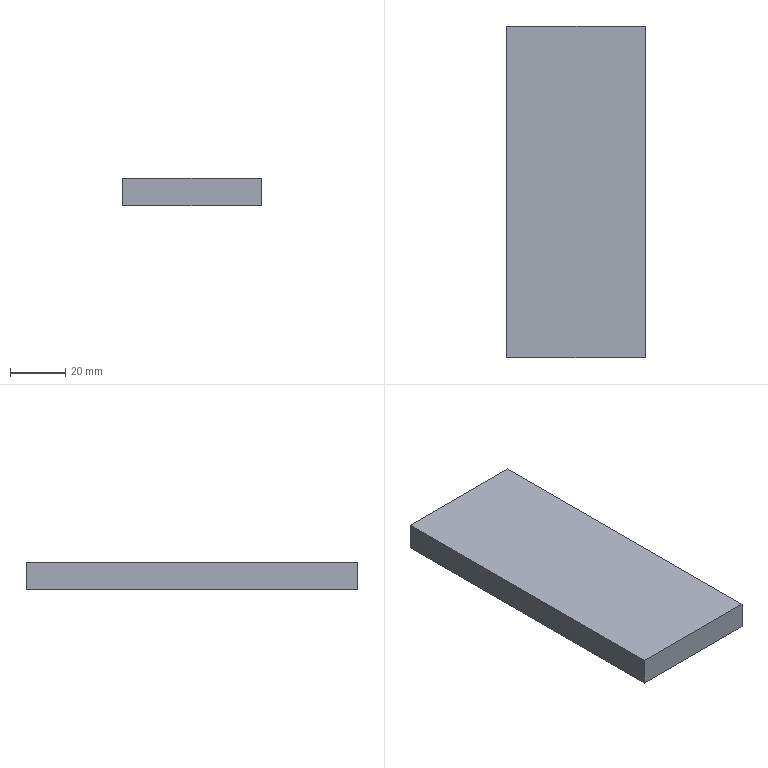Part | SolidWorks | features Extrusion 1 | 1 solid | 6 faces | box 50 x 120 x 10 mm | volume 60000 mm3 | plane 6
STEP:
#1=CARTESIAN_POINT('',(-25.,60.,-5.));
#2=VERTEX_POINT('',#1);
#3=CARTESIAN_POINT('',(-25.,-60.,-5.));
#4=VERTEX_POINT('',#3);
#5=CARTESIAN_POINT('',(-25.,60.,-5.));
#6=DIRECTION('',(0.,-1.,0.));
#7=VECTOR('',#6,1000.);
#8=LINE('',#5,#7);
#9=EDGE_CURVE('',#2,#4,#8,.T.);
#10=ORIENTED_EDGE('',*,*,#9,.T.);
#11=CARTESIAN_POINT('',(-25.,-60.,5.));
#12=VERTEX_POINT('',#11);
#13=CARTESIAN_POINT('',(-25.,-60.,5.));
#14=DIRECTION('',(0.,0.,-1.));
#15=VECTOR('',#14,1000.);
#16=LINE('',#13,#15);
#17=EDGE_CURVE('',#12,#4,#16,.T.);
#18=ORIENTED_EDGE('',*,*,#17,.F.);
#19=CARTESIAN_POINT('',(-25.,60.,5.));
#20=VERTEX_POINT('',#19);
#21=CARTESIAN_POINT('',(-25.,60.,5.));
#22=DIRECTION('',(0.,-1.,0.));
#23=VECTOR('',#22,1000.);
#24=LINE('',#21,#23);
#25=EDGE_CURVE('',#20,#12,#24,.T.);
#26=ORIENTED_EDGE('',*,*,#25,.F.);
#27=CARTESIAN_POINT('',(-25.,60.,5.));
#28=DIRECTION('',(0.,0.,-1.));
#29=VECTOR('',#28,1000.);
#30=LINE('',#27,#29);
#31=EDGE_CURVE('',#20,#2,#30,.T.);
#32=ORIENTED_EDGE('',*,*,#31,.T.);
#33=EDGE_LOOP('',(#10,#18,#26,#32));
#34=FACE_OUTER_BOUND('',#33,.T.);
#35=CARTESIAN_POINT('',(-25.,60.,5.));
#36=DIRECTION('',(1.,0.,0.));
#37=DIRECTION('',(0.,1.,0.));
#38=AXIS2_PLACEMENT_3D('',#35,#36,#37);
#39=PLANE('',#38);
#40=ADVANCED_FACE('',(#34),#39,.F.);
#41=CARTESIAN_POINT('',(25.,-60.,-5.));
#42=VERTEX_POINT('',#41);
#43=CARTESIAN_POINT('',(-25.,-60.,-5.));
#44=DIRECTION('',(1.,0.,0.));
#45=VECTOR('',#44,1000.);
#46=LINE('',#43,#45);
#47=EDGE_CURVE('',#4,#42,#46,.T.);
#48=ORIENTED_EDGE('',*,*,#47,.T.);
#49=CARTESIAN_POINT('',(25.,-60.,5.));
#50=VERTEX_POINT('',#49);
#51=CARTESIAN_POINT('',(25.,-60.,5.));
#52=DIRECTION('',(0.,0.,-1.));
#53=VECTOR('',#52,1000.);
#54=LINE('',#51,#53);
#55=EDGE_CURVE('',#50,#42,#54,.T.);
#56=ORIENTED_EDGE('',*,*,#55,.F.);
#57=CARTESIAN_POINT('',(-25.,-60.,5.));
#58=DIRECTION('',(1.,0.,0.));
#59=VECTOR('',#58,1000.);
#60=LINE('',#57,#59);
#61=EDGE_CURVE('',#12,#50,#60,.T.);
#62=ORIENTED_EDGE('',*,*,#61,.F.);
#63=ORIENTED_EDGE('',*,*,#17,.T.);
#64=EDGE_LOOP('',(#48,#56,#62,#63));
#65=FACE_OUTER_BOUND('',#64,.T.);
#66=CARTESIAN_POINT('',(-25.,-60.,5.));
#67=DIRECTION('',(0.,1.,0.));
#68=DIRECTION('',(0.,0.,1.));
#69=AXIS2_PLACEMENT_3D('',#66,#67,#68);
#70=PLANE('',#69);
#71=ADVANCED_FACE('',(#65),#70,.F.);
#72=CARTESIAN_POINT('',(25.,60.,-5.));
#73=VERTEX_POINT('',#72);
#74=CARTESIAN_POINT('',(25.,60.,-5.));
#75=DIRECTION('',(0.,1.,0.));
#76=VECTOR('',#75,1000.);
#77=LINE('',#74,#76);
#78=EDGE_CURVE('',#42,#73,#77,.T.);
#79=ORIENTED_EDGE('',*,*,#78,.T.);
#80=CARTESIAN_POINT('',(25.,60.,5.));
#81=VERTEX_POINT('',#80);
#82=CARTESIAN_POINT('',(25.,60.,5.));
#83=DIRECTION('',(0.,0.,-1.));
#84=VECTOR('',#83,1000.);
#85=LINE('',#82,#84);
#86=EDGE_CURVE('',#81,#73,#85,.T.);
#87=ORIENTED_EDGE('',*,*,#86,.F.);
#88=CARTESIAN_POINT('',(25.,60.,5.));
#89=DIRECTION('',(0.,1.,0.));
#90=VECTOR('',#89,1000.);
#91=LINE('',#88,#90);
#92=EDGE_CURVE('',#50,#81,#91,.T.);
#93=ORIENTED_EDGE('',*,*,#92,.F.);
#94=ORIENTED_EDGE('',*,*,#55,.T.);
#95=EDGE_LOOP('',(#79,#87,#93,#94));
#96=FACE_OUTER_BOUND('',#95,.T.);
#97=CARTESIAN_POINT('',(25.,60.,5.));
#98=DIRECTION('',(-1.,0.,0.));
#99=DIRECTION('',(0.,-1.,0.));
#100=AXIS2_PLACEMENT_3D('',#97,#98,#99);
#101=PLANE('',#100);
#102=ADVANCED_FACE('',(#96),#101,.F.);
#103=CARTESIAN_POINT('',(-25.,60.,-5.));
#104=DIRECTION('',(-1.,0.,0.));
#105=VECTOR('',#104,1000.);
#106=LINE('',#103,#105);
#107=EDGE_CURVE('',#73,#2,#106,.T.);
#108=ORIENTED_EDGE('',*,*,#107,.T.);
#109=ORIENTED_EDGE('',*,*,#31,.F.);
#110=CARTESIAN_POINT('',(-25.,60.,5.));
#111=DIRECTION('',(-1.,0.,0.));
#112=VECTOR('',#111,1000.);
#113=LINE('',#110,#112);
#114=EDGE_CURVE('',#81,#20,#113,.T.);
#115=ORIENTED_EDGE('',*,*,#114,.F.);
#116=ORIENTED_EDGE('',*,*,#86,.T.);
#117=EDGE_LOOP('',(#108,#109,#115,#116));
#118=FACE_OUTER_BOUND('',#117,.T.);
#119=CARTESIAN_POINT('',(-25.,60.,5.));
#120=DIRECTION('',(0.,-1.,0.));
#121=DIRECTION('',(0.,0.,-1.));
#122=AXIS2_PLACEMENT_3D('',#119,#120,#121);
#123=PLANE('',#122);
#124=ADVANCED_FACE('',(#118),#123,.F.);
#125=ORIENTED_EDGE('',*,*,#25,.T.);
#126=ORIENTED_EDGE('',*,*,#61,.T.);
#127=ORIENTED_EDGE('',*,*,#92,.T.);
#128=ORIENTED_EDGE('',*,*,#114,.T.);
#129=EDGE_LOOP('',(#125,#126,#127,#128));
#130=FACE_OUTER_BOUND('',#129,.T.);
#131=CARTESIAN_POINT('',(-25.,-60.,5.));
#132=DIRECTION('',(0.,0.,1.));
#133=DIRECTION('',(1.,0.,0.));
#134=AXIS2_PLACEMENT_3D('',#131,#132,#133);
#135=PLANE('',#134);
#136=ADVANCED_FACE('',(#130),#135,.T.);
#137=ORIENTED_EDGE('',*,*,#9,.F.);
#138=ORIENTED_EDGE('',*,*,#107,.F.);
#139=ORIENTED_EDGE('',*,*,#78,.F.);
#140=ORIENTED_EDGE('',*,*,#47,.F.);
#141=EDGE_LOOP('',(#137,#138,#139,#140));
#142=FACE_OUTER_BOUND('',#141,.T.);
#143=CARTESIAN_POINT('',(-25.,-60.,-5.));
#144=DIRECTION('',(0.,0.,1.));
#145=DIRECTION('',(1.,0.,0.));
#146=AXIS2_PLACEMENT_3D('',#143,#144,#145);
#147=PLANE('',#146);
#148=ADVANCED_FACE('',(#142),#147,.F.);
#149=CLOSED_SHELL('',(#40,#71,#102,#124,#136,#148));
#150=MANIFOLD_SOLID_BREP('',#149);
#151=CARTESIAN_POINT('',(0.,0.,0.));
#152=DIRECTION('',(0.,0.,1.));
#153=DIRECTION('',(1.,0.,0.));
#154=AXIS2_PLACEMENT_3D('',#151,#152,#153);
#155=(LENGTH_UNIT()NAMED_UNIT(*)SI_UNIT(.MILLI.,.METRE.));
#156=UNCERTAINTY_MEASURE_WITH_UNIT(LENGTH_MEASURE(0.00001),#155,'','');
#157=(NAMED_UNIT(*)PLANE_ANGLE_UNIT()SI_UNIT($,.RADIAN.));
#158=(NAMED_UNIT(*)SI_UNIT($,.STERADIAN.)SOLID_ANGLE_UNIT());
#159=(GEOMETRIC_REPRESENTATION_CONTEXT(3)GLOBAL_UNCERTAINTY_ASSIGNED_CONTEXT((#156))GLOBAL_UNIT_ASSIGNED_CONTEXT((#155,#157,#158))REPRESENTATION_CONTEXT('',''));
#160=ADVANCED_BREP_SHAPE_REPRESENTATION('',(#150,#154),#159);